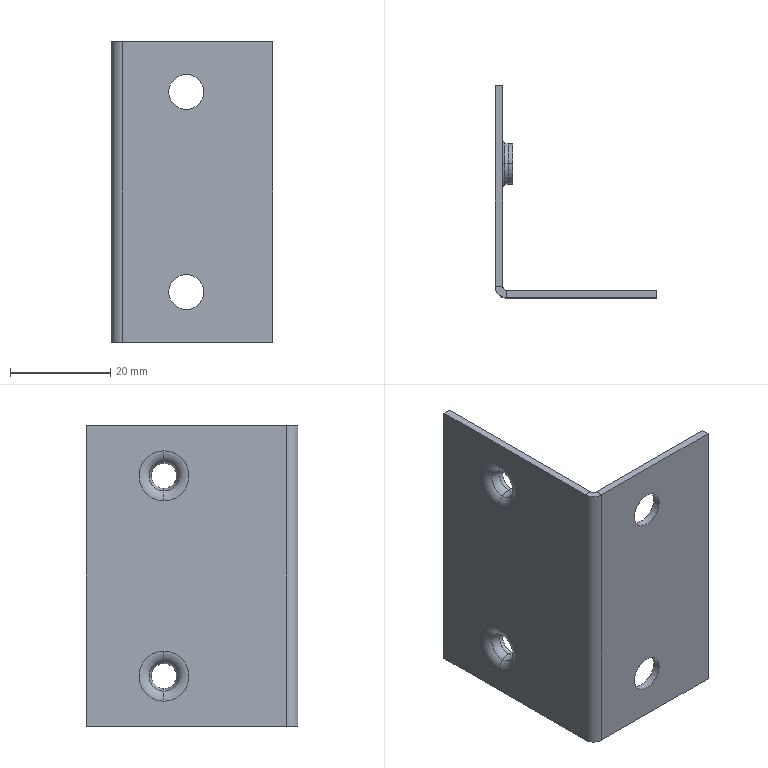Part | STEP file | 68332991 | 1 solid | 46 faces | box 32.3 x 42.3 x 60 mm | volume 6427 mm3 | plane 16 | torus 16 | cylinder 14 | commonest cylinder face diameters 5 x4 7 x4 8 x4 1.6 x1 4.6 x1